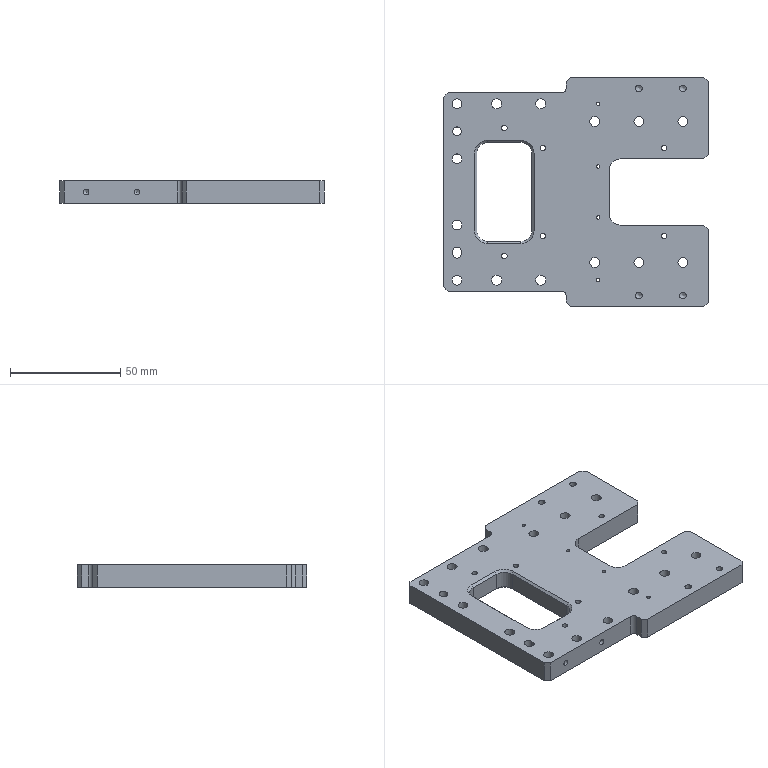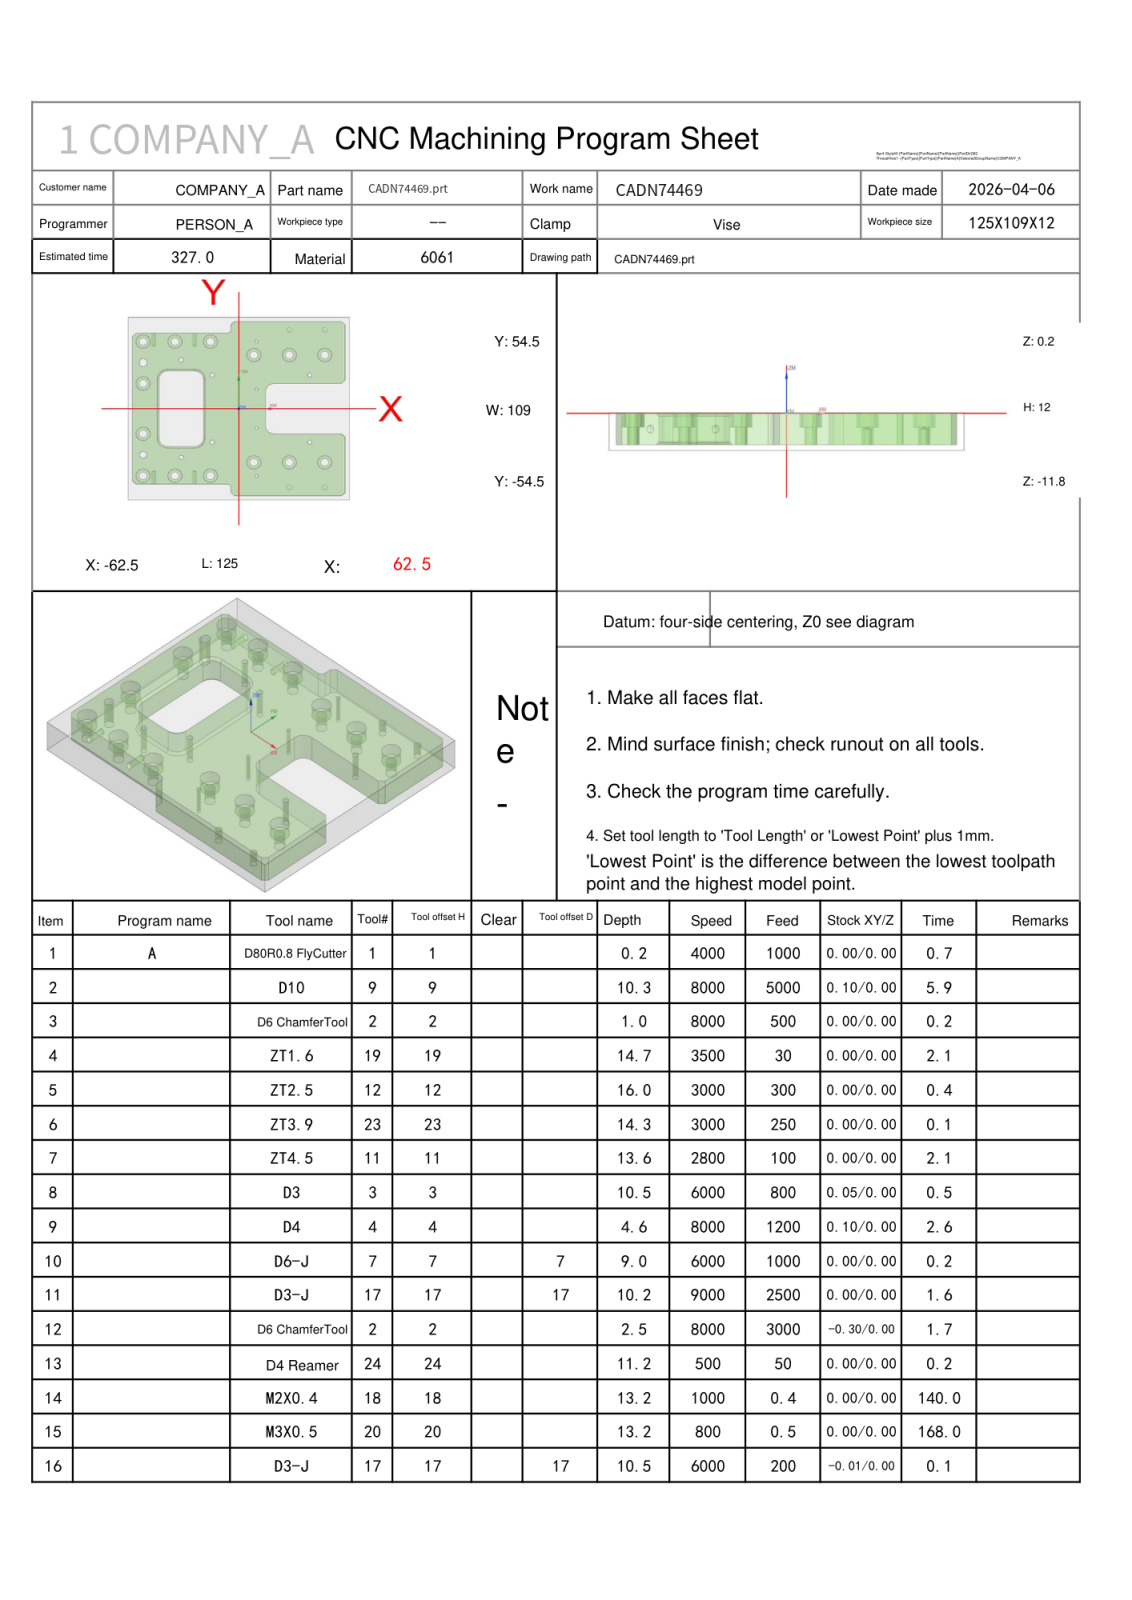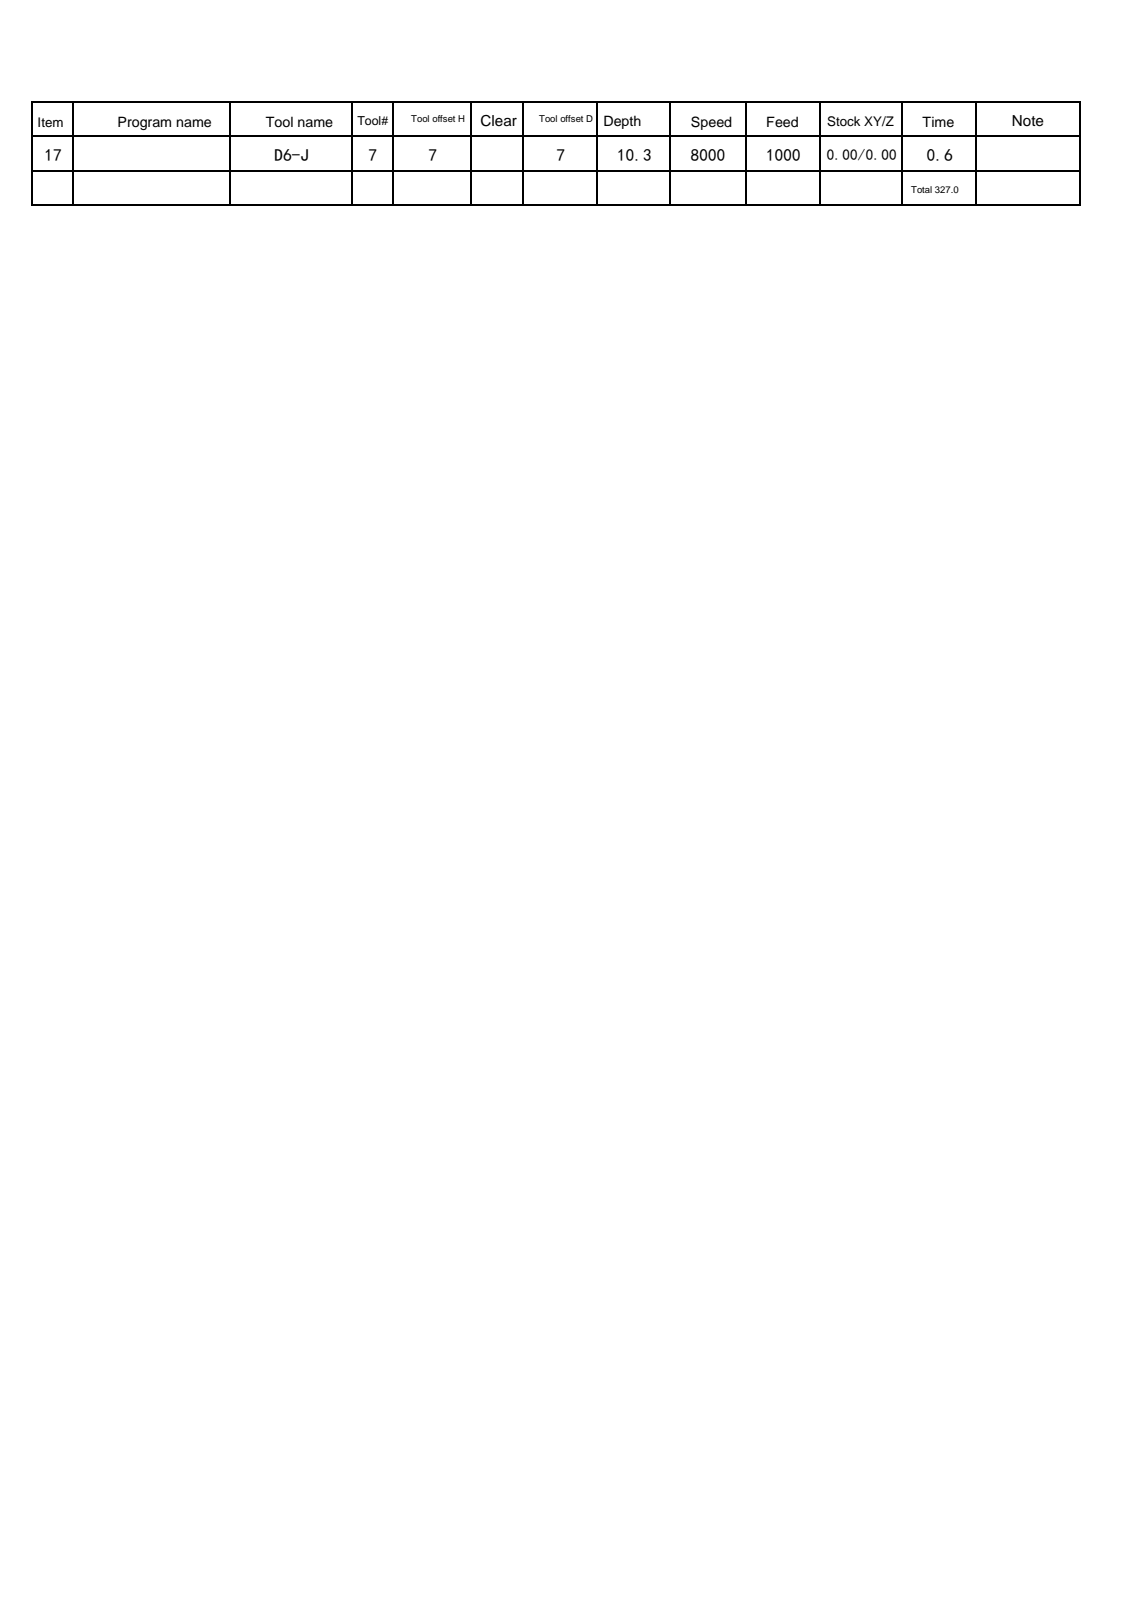NC program | NX | posted by the shop | part box 120 x 104 x 10 mm
Lines 1 to 44 of 6435:
%
O0001
(Machine time: 616.16 MIN)
(===Total Tool:14===)
(T1=D80R0.8 FlyCutter D=80.  R=0.8  D-  H01 Z=0.    )
(T9=D10     D=10.  R=0.   D-  H09 Z=-10.1 )
(T2=D6 ChamferTool   D=6.   R=0.   D-  H02 Z=-2.3  )
(T19=ZT1.6  D=1.6  DR_a=118 D-  H19 Z=-14.48)
(T12=ZT2.5  D=2.5  DR_a=118 D-  H12 Z=-15.75)
(T23=ZT3.9  D=3.9  DR_a=120 D-  H23 Z=-14.13)
(T11=ZT4.5  D=4.5  DR_a=118 D-  H11 Z=-13.35)
(T3=D3      D=3.   R=0.   D-  H03 Z=-10.3 )
(T4=D4      D=4.   R=0.   D-  H04 Z=-4.4  )
(T7=D6-J    D=6.   R=0.   D7  H07 Z=-10.1 )
(T17=D3-J   D=3.   R=0.   D17 H17 Z=-10.3 )
(T24=D4 Reamer   D=4.   DR_a=180 D-  H24 Z=-11.  )
(T18=M2X0.4 D=1.6  DR_a=180 D-  H18 Z=-13.  )
(T20=M3X0.5 D=2.5  DR_a=180 D-  H20 Z=-13.  )
G80 G90 G17 G49 G40
G91 G28 Z0
M01
N1 T01 M06
(D80R0.8 FlyCutter  D=80. R=0.8 H=01 ce=0.00 di=0.00)
G00 G90 G54 X105. Y-46. M03 S4000
G43 H01 Z20.
M08
Z2.
G01 Z0.0 F1000.
X100.
X-100.
Y0.0
X100.
Y46.
X-100.
X-105.
Z2.
G00 Z20.
G91 G28 Z0.0
M05
M09
G91 G28 Z0.0
M01